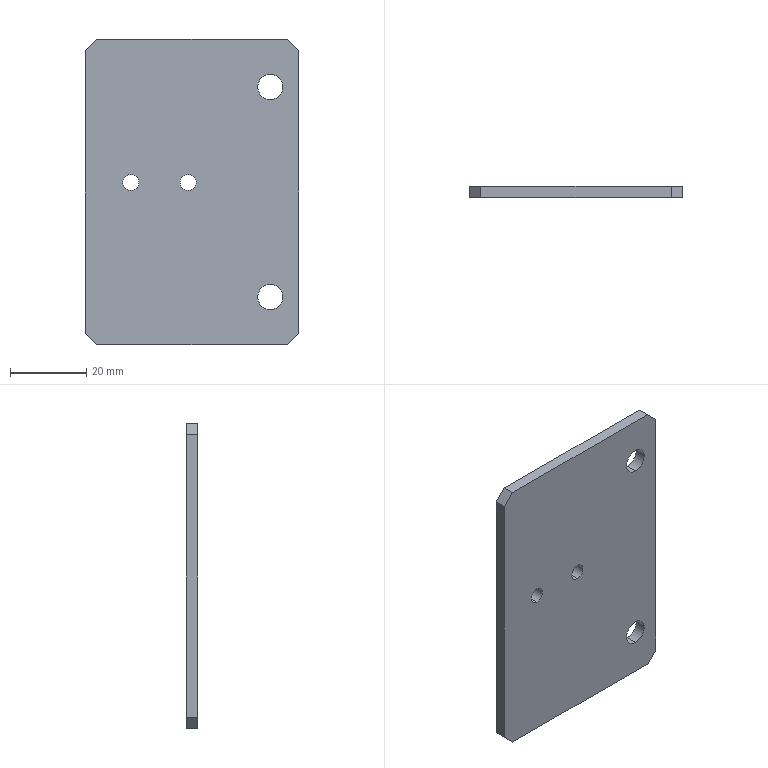Part | STEP file | 11-FG-SJ01311 | 1 solid | 18 faces | box 56 x 3 x 80 mm | volume 13098 mm3 | plane 10 | cylinder 8 | commonest cylinder face diameters 4.2 x4 6.6 x4
STEP:
#1=CARTESIAN_POINT('',(12.,50.,40.4));
#2=VERTEX_POINT('',#1);
#3=CARTESIAN_POINT('',(12.,50.,44.6));
#4=VERTEX_POINT('',#3);
#5=CARTESIAN_POINT('',(12.,50.,42.5));
#6=DIRECTION('',(0.,1.,0.));
#7=DIRECTION('',(0.,0.,1.));
#8=AXIS2_PLACEMENT_3D('',#5,#6,#7);
#9=CIRCLE('',#8,2.1);
#10=EDGE_CURVE('',#2,#4,#9,.T.);
#11=ORIENTED_EDGE('',*,*,#10,.T.);
#12=CARTESIAN_POINT('',(12.,47.,44.6));
#13=VERTEX_POINT('',#12);
#14=CARTESIAN_POINT('',(12.,47.,44.6));
#15=DIRECTION('',(0.,-1.,0.));
#16=VECTOR('',#15,1000.);
#17=LINE('',#14,#16);
#18=EDGE_CURVE('',#4,#13,#17,.T.);
#19=ORIENTED_EDGE('',*,*,#18,.T.);
#20=CARTESIAN_POINT('',(12.,47.,40.4));
#21=VERTEX_POINT('',#20);
#22=CARTESIAN_POINT('',(12.,47.,42.5));
#23=DIRECTION('',(0.,-1.,0.));
#24=DIRECTION('',(0.,0.,-1.));
#25=AXIS2_PLACEMENT_3D('',#22,#23,#24);
#26=CIRCLE('',#25,2.1);
#27=EDGE_CURVE('',#13,#21,#26,.T.);
#28=ORIENTED_EDGE('',*,*,#27,.T.);
#29=CARTESIAN_POINT('',(12.,47.,40.4));
#30=DIRECTION('',(0.,-1.,0.));
#31=VECTOR('',#30,1000.);
#32=LINE('',#29,#31);
#33=EDGE_CURVE('',#2,#21,#32,.T.);
#34=ORIENTED_EDGE('',*,*,#33,.F.);
#35=EDGE_LOOP('',(#11,#19,#28,#34));
#36=FACE_OUTER_BOUND('',#35,.T.);
#37=CARTESIAN_POINT('',(12.,47.,42.5));
#38=DIRECTION('',(0.,-1.,0.));
#39=DIRECTION('',(0.,0.,-1.));
#40=AXIS2_PLACEMENT_3D('',#37,#38,#39);
#41=CYLINDRICAL_SURFACE('',#40,2.1);
#42=ADVANCED_FACE('',(#36),#41,.F.);
#43=CARTESIAN_POINT('',(27.,50.,40.4));
#44=VERTEX_POINT('',#43);
#45=CARTESIAN_POINT('',(27.,50.,44.6));
#46=VERTEX_POINT('',#45);
#47=CARTESIAN_POINT('',(27.,50.,42.5));
#48=DIRECTION('',(0.,1.,0.));
#49=DIRECTION('',(0.,0.,1.));
#50=AXIS2_PLACEMENT_3D('',#47,#48,#49);
#51=CIRCLE('',#50,2.1);
#52=EDGE_CURVE('',#44,#46,#51,.T.);
#53=ORIENTED_EDGE('',*,*,#52,.T.);
#54=CARTESIAN_POINT('',(27.,47.,44.6));
#55=VERTEX_POINT('',#54);
#56=CARTESIAN_POINT('',(27.,47.,44.6));
#57=DIRECTION('',(0.,-1.,0.));
#58=VECTOR('',#57,1000.);
#59=LINE('',#56,#58);
#60=EDGE_CURVE('',#46,#55,#59,.T.);
#61=ORIENTED_EDGE('',*,*,#60,.T.);
#62=CARTESIAN_POINT('',(27.,47.,40.4));
#63=VERTEX_POINT('',#62);
#64=CARTESIAN_POINT('',(27.,47.,42.5));
#65=DIRECTION('',(0.,-1.,0.));
#66=DIRECTION('',(0.,0.,-1.));
#67=AXIS2_PLACEMENT_3D('',#64,#65,#66);
#68=CIRCLE('',#67,2.1);
#69=EDGE_CURVE('',#55,#63,#68,.T.);
#70=ORIENTED_EDGE('',*,*,#69,.T.);
#71=CARTESIAN_POINT('',(27.,47.,40.4));
#72=DIRECTION('',(0.,-1.,0.));
#73=VECTOR('',#72,1000.);
#74=LINE('',#71,#73);
#75=EDGE_CURVE('',#44,#63,#74,.T.);
#76=ORIENTED_EDGE('',*,*,#75,.F.);
#77=EDGE_LOOP('',(#53,#61,#70,#76));
#78=FACE_OUTER_BOUND('',#77,.T.);
#79=CARTESIAN_POINT('',(27.,47.,42.5));
#80=DIRECTION('',(0.,-1.,0.));
#81=DIRECTION('',(0.,0.,-1.));
#82=AXIS2_PLACEMENT_3D('',#79,#80,#81);
#83=CYLINDRICAL_SURFACE('',#82,2.1);
#84=ADVANCED_FACE('',(#78),#83,.F.);
#85=CARTESIAN_POINT('',(48.5,50.,70.8));
#86=VERTEX_POINT('',#85);
#87=CARTESIAN_POINT('',(48.5,50.,64.2));
#88=VERTEX_POINT('',#87);
#89=CARTESIAN_POINT('',(48.5,50.,67.5));
#90=DIRECTION('',(0.,-1.,0.));
#91=DIRECTION('',(0.,0.,-1.));
#92=AXIS2_PLACEMENT_3D('',#89,#90,#91);
#93=CIRCLE('',#92,3.3);
#94=EDGE_CURVE('',#86,#88,#93,.T.);
#95=ORIENTED_EDGE('',*,*,#94,.F.);
#96=CARTESIAN_POINT('',(48.5,47.,70.8));
#97=VERTEX_POINT('',#96);
#98=CARTESIAN_POINT('',(48.5,47.,70.8));
#99=DIRECTION('',(0.,-1.,0.));
#100=VECTOR('',#99,1000.);
#101=LINE('',#98,#100);
#102=EDGE_CURVE('',#86,#97,#101,.T.);
#103=ORIENTED_EDGE('',*,*,#102,.T.);
#104=CARTESIAN_POINT('',(48.5,47.,64.2));
#105=VERTEX_POINT('',#104);
#106=CARTESIAN_POINT('',(48.5,47.,67.5));
#107=DIRECTION('',(0.,-1.,0.));
#108=DIRECTION('',(0.,0.,-1.));
#109=AXIS2_PLACEMENT_3D('',#106,#107,#108);
#110=CIRCLE('',#109,3.3);
#111=EDGE_CURVE('',#97,#105,#110,.T.);
#112=ORIENTED_EDGE('',*,*,#111,.T.);
#113=CARTESIAN_POINT('',(48.5,47.,64.2));
#114=DIRECTION('',(0.,-1.,0.));
#115=VECTOR('',#114,1000.);
#116=LINE('',#113,#115);
#117=EDGE_CURVE('',#88,#105,#116,.T.);
#118=ORIENTED_EDGE('',*,*,#117,.F.);
#119=EDGE_LOOP('',(#95,#103,#112,#118));
#120=FACE_OUTER_BOUND('',#119,.T.);
#121=CARTESIAN_POINT('',(48.5,47.,67.5));
#122=DIRECTION('',(0.,-1.,0.));
#123=DIRECTION('',(0.,0.,-1.));
#124=AXIS2_PLACEMENT_3D('',#121,#122,#123);
#125=CYLINDRICAL_SURFACE('',#124,3.3);
#126=ADVANCED_FACE('',(#120),#125,.F.);
#127=CARTESIAN_POINT('',(48.5,50.,15.8));
#128=VERTEX_POINT('',#127);
#129=CARTESIAN_POINT('',(48.5,50.,9.2));
#130=VERTEX_POINT('',#129);
#131=CARTESIAN_POINT('',(48.5,50.,12.5));
#132=DIRECTION('',(0.,-1.,0.));
#133=DIRECTION('',(0.,0.,-1.));
#134=AXIS2_PLACEMENT_3D('',#131,#132,#133);
#135=CIRCLE('',#134,3.3);
#136=EDGE_CURVE('',#128,#130,#135,.T.);
#137=ORIENTED_EDGE('',*,*,#136,.F.);
#138=CARTESIAN_POINT('',(48.5,47.,15.8));
#139=VERTEX_POINT('',#138);
#140=CARTESIAN_POINT('',(48.5,47.,15.8));
#141=DIRECTION('',(0.,-1.,0.));
#142=VECTOR('',#141,1000.);
#143=LINE('',#140,#142);
#144=EDGE_CURVE('',#128,#139,#143,.T.);
#145=ORIENTED_EDGE('',*,*,#144,.T.);
#146=CARTESIAN_POINT('',(48.5,47.,9.2));
#147=VERTEX_POINT('',#146);
#148=CARTESIAN_POINT('',(48.5,47.,12.5));
#149=DIRECTION('',(0.,-1.,0.));
#150=DIRECTION('',(0.,0.,-1.));
#151=AXIS2_PLACEMENT_3D('',#148,#149,#150);
#152=CIRCLE('',#151,3.3);
#153=EDGE_CURVE('',#139,#147,#152,.T.);
#154=ORIENTED_EDGE('',*,*,#153,.T.);
#155=CARTESIAN_POINT('',(48.5,47.,9.2));
#156=DIRECTION('',(0.,-1.,0.));
#157=VECTOR('',#156,1000.);
#158=LINE('',#155,#157);
#159=EDGE_CURVE('',#130,#147,#158,.T.);
#160=ORIENTED_EDGE('',*,*,#159,.F.);
#161=EDGE_LOOP('',(#137,#145,#154,#160));
#162=FACE_OUTER_BOUND('',#161,.T.);
#163=CARTESIAN_POINT('',(48.5,47.,12.5));
#164=DIRECTION('',(0.,-1.,0.));
#165=DIRECTION('',(0.,0.,-1.));
#166=AXIS2_PLACEMENT_3D('',#163,#164,#165);
#167=CYLINDRICAL_SURFACE('',#166,3.3);
#168=ADVANCED_FACE('',(#162),#167,.F.);
#169=CARTESIAN_POINT('',(12.,47.,42.5));
#170=DIRECTION('',(0.,-1.,0.));
#171=DIRECTION('',(0.,0.,-1.));
#172=AXIS2_PLACEMENT_3D('',#169,#170,#171);
#173=CIRCLE('',#172,2.1);
#174=EDGE_CURVE('',#21,#13,#173,.T.);
#175=ORIENTED_EDGE('',*,*,#174,.F.);
#176=ORIENTED_EDGE('',*,*,#27,.F.);
#177=EDGE_LOOP('',(#175,#176));
#178=FACE_BOUND('',#177,.T.);
#179=CARTESIAN_POINT('',(27.,47.,42.5));
#180=DIRECTION('',(0.,-1.,0.));
#181=DIRECTION('',(0.,0.,-1.));
#182=AXIS2_PLACEMENT_3D('',#179,#180,#181);
#183=CIRCLE('',#182,2.1);
#184=EDGE_CURVE('',#63,#55,#183,.T.);
#185=ORIENTED_EDGE('',*,*,#184,.F.);
#186=ORIENTED_EDGE('',*,*,#69,.F.);
#187=EDGE_LOOP('',(#185,#186));
#188=FACE_BOUND('',#187,.T.);
#189=CARTESIAN_POINT('',(48.5,47.,67.5));
#190=DIRECTION('',(0.,-1.,0.));
#191=DIRECTION('',(0.,0.,-1.));
#192=AXIS2_PLACEMENT_3D('',#189,#190,#191);
#193=CIRCLE('',#192,3.3);
#194=EDGE_CURVE('',#105,#97,#193,.T.);
#195=ORIENTED_EDGE('',*,*,#194,.F.);
#196=ORIENTED_EDGE('',*,*,#111,.F.);
#197=EDGE_LOOP('',(#195,#196));
#198=FACE_BOUND('',#197,.T.);
#199=CARTESIAN_POINT('',(48.5,47.,12.5));
#200=DIRECTION('',(0.,-1.,0.));
#201=DIRECTION('',(0.,0.,-1.));
#202=AXIS2_PLACEMENT_3D('',#199,#200,#201);
#203=CIRCLE('',#202,3.3);
#204=EDGE_CURVE('',#147,#139,#203,.T.);
#205=ORIENTED_EDGE('',*,*,#204,.F.);
#206=ORIENTED_EDGE('',*,*,#153,.F.);
#207=EDGE_LOOP('',(#205,#206));
#208=FACE_BOUND('',#207,.T.);
#209=CARTESIAN_POINT('',(0.,47.,77.));
#210=VERTEX_POINT('',#209);
#211=CARTESIAN_POINT('',(0.,47.,3.));
#212=VERTEX_POINT('',#211);
#213=CARTESIAN_POINT('',(0.,47.,80.));
#214=DIRECTION('',(0.,0.,-1.));
#215=VECTOR('',#214,1000.);
#216=LINE('',#213,#215);
#217=EDGE_CURVE('',#210,#212,#216,.T.);
#218=ORIENTED_EDGE('',*,*,#217,.T.);
#219=CARTESIAN_POINT('',(3.,47.,0.));
#220=VERTEX_POINT('',#219);
#221=CARTESIAN_POINT('',(3.,47.,0.));
#222=DIRECTION('',(0.7071,0.,-0.7071));
#223=VECTOR('',#222,1000.);
#224=LINE('',#221,#223);
#225=EDGE_CURVE('',#212,#220,#224,.T.);
#226=ORIENTED_EDGE('',*,*,#225,.T.);
#227=CARTESIAN_POINT('',(53.,47.,0.));
#228=VERTEX_POINT('',#227);
#229=CARTESIAN_POINT('',(0.,47.,0.));
#230=DIRECTION('',(1.,0.,0.));
#231=VECTOR('',#230,1000.);
#232=LINE('',#229,#231);
#233=EDGE_CURVE('',#220,#228,#232,.T.);
#234=ORIENTED_EDGE('',*,*,#233,.T.);
#235=CARTESIAN_POINT('',(56.,47.,3.));
#236=VERTEX_POINT('',#235);
#237=CARTESIAN_POINT('',(53.,47.,0.));
#238=DIRECTION('',(0.7071,0.,0.7071));
#239=VECTOR('',#238,1000.);
#240=LINE('',#237,#239);
#241=EDGE_CURVE('',#228,#236,#240,.T.);
#242=ORIENTED_EDGE('',*,*,#241,.T.);
#243=CARTESIAN_POINT('',(56.,47.,77.));
#244=VERTEX_POINT('',#243);
#245=CARTESIAN_POINT('',(56.,47.,80.));
#246=DIRECTION('',(0.,0.,-1.));
#247=VECTOR('',#246,1000.);
#248=LINE('',#245,#247);
#249=EDGE_CURVE('',#244,#236,#248,.T.);
#250=ORIENTED_EDGE('',*,*,#249,.F.);
#251=CARTESIAN_POINT('',(53.,47.,80.));
#252=VERTEX_POINT('',#251);
#253=CARTESIAN_POINT('',(56.,47.,77.));
#254=DIRECTION('',(-0.7071,0.,0.7071));
#255=VECTOR('',#254,1000.);
#256=LINE('',#253,#255);
#257=EDGE_CURVE('',#244,#252,#256,.T.);
#258=ORIENTED_EDGE('',*,*,#257,.T.);
#259=CARTESIAN_POINT('',(3.,47.,80.));
#260=VERTEX_POINT('',#259);
#261=CARTESIAN_POINT('',(0.,47.,80.));
#262=DIRECTION('',(1.,0.,0.));
#263=VECTOR('',#262,1000.);
#264=LINE('',#261,#263);
#265=EDGE_CURVE('',#260,#252,#264,.T.);
#266=ORIENTED_EDGE('',*,*,#265,.F.);
#267=CARTESIAN_POINT('',(0.,47.,77.));
#268=DIRECTION('',(-0.7071,0.,-0.7071));
#269=VECTOR('',#268,1000.);
#270=LINE('',#267,#269);
#271=EDGE_CURVE('',#260,#210,#270,.T.);
#272=ORIENTED_EDGE('',*,*,#271,.T.);
#273=EDGE_LOOP('',(#218,#226,#234,#242,#250,#258,#266,#272));
#274=FACE_OUTER_BOUND('',#273,.T.);
#275=CARTESIAN_POINT('',(0.,47.,80.));
#276=DIRECTION('',(0.,1.,0.));
#277=DIRECTION('',(0.,0.,1.));
#278=AXIS2_PLACEMENT_3D('',#275,#276,#277);
#279=PLANE('',#278);
#280=ADVANCED_FACE('',(#178,#188,#198,#208,#274),#279,.F.);
#281=ORIENTED_EDGE('',*,*,#249,.T.);
#282=CARTESIAN_POINT('',(56.,50.,3.));
#283=VERTEX_POINT('',#282);
#284=CARTESIAN_POINT('',(56.,50.,3.));
#285=DIRECTION('',(0.,1.,0.));
#286=VECTOR('',#285,1000.);
#287=LINE('',#284,#286);
#288=EDGE_CURVE('',#236,#283,#287,.T.);
#289=ORIENTED_EDGE('',*,*,#288,.T.);
#290=CARTESIAN_POINT('',(56.,50.,77.));
#291=VERTEX_POINT('',#290);
#292=CARTESIAN_POINT('',(56.,50.,80.));
#293=DIRECTION('',(0.,0.,-1.));
#294=VECTOR('',#293,1000.);
#295=LINE('',#292,#294);
#296=EDGE_CURVE('',#291,#283,#295,.T.);
#297=ORIENTED_EDGE('',*,*,#296,.F.);
#298=CARTESIAN_POINT('',(56.,47.,77.));
#299=DIRECTION('',(0.,-1.,0.));
#300=VECTOR('',#299,1000.);
#301=LINE('',#298,#300);
#302=EDGE_CURVE('',#291,#244,#301,.T.);
#303=ORIENTED_EDGE('',*,*,#302,.T.);
#304=EDGE_LOOP('',(#281,#289,#297,#303));
#305=FACE_OUTER_BOUND('',#304,.T.);
#306=CARTESIAN_POINT('',(56.,50.,80.));
#307=DIRECTION('',(1.,0.,0.));
#308=DIRECTION('',(0.,0.,-1.));
#309=AXIS2_PLACEMENT_3D('',#306,#307,#308);
#310=PLANE('',#309);
#311=ADVANCED_FACE('',(#305),#310,.T.);
#312=ORIENTED_EDGE('',*,*,#10,.F.);
#313=CARTESIAN_POINT('',(12.,50.,42.5));
#314=DIRECTION('',(0.,1.,0.));
#315=DIRECTION('',(0.,0.,1.));
#316=AXIS2_PLACEMENT_3D('',#313,#314,#315);
#317=CIRCLE('',#316,2.1);
#318=EDGE_CURVE('',#4,#2,#317,.T.);
#319=ORIENTED_EDGE('',*,*,#318,.F.);
#320=EDGE_LOOP('',(#312,#319));
#321=FACE_BOUND('',#320,.T.);
#322=ORIENTED_EDGE('',*,*,#52,.F.);
#323=CARTESIAN_POINT('',(27.,50.,42.5));
#324=DIRECTION('',(0.,1.,0.));
#325=DIRECTION('',(0.,0.,1.));
#326=AXIS2_PLACEMENT_3D('',#323,#324,#325);
#327=CIRCLE('',#326,2.1);
#328=EDGE_CURVE('',#46,#44,#327,.T.);
#329=ORIENTED_EDGE('',*,*,#328,.F.);
#330=EDGE_LOOP('',(#322,#329));
#331=FACE_BOUND('',#330,.T.);
#332=CARTESIAN_POINT('',(48.5,50.,67.5));
#333=DIRECTION('',(0.,-1.,0.));
#334=DIRECTION('',(0.,0.,-1.));
#335=AXIS2_PLACEMENT_3D('',#332,#333,#334);
#336=CIRCLE('',#335,3.3);
#337=EDGE_CURVE('',#88,#86,#336,.T.);
#338=ORIENTED_EDGE('',*,*,#337,.T.);
#339=ORIENTED_EDGE('',*,*,#94,.T.);
#340=EDGE_LOOP('',(#338,#339));
#341=FACE_BOUND('',#340,.T.);
#342=CARTESIAN_POINT('',(48.5,50.,12.5));
#343=DIRECTION('',(0.,-1.,0.));
#344=DIRECTION('',(0.,0.,-1.));
#345=AXIS2_PLACEMENT_3D('',#342,#343,#344);
#346=CIRCLE('',#345,3.3);
#347=EDGE_CURVE('',#130,#128,#346,.T.);
#348=ORIENTED_EDGE('',*,*,#347,.T.);
#349=ORIENTED_EDGE('',*,*,#136,.T.);
#350=EDGE_LOOP('',(#348,#349));
#351=FACE_BOUND('',#350,.T.);
#352=CARTESIAN_POINT('',(3.,50.,0.));
#353=VERTEX_POINT('',#352);
#354=CARTESIAN_POINT('',(53.,50.,0.));
#355=VERTEX_POINT('',#354);
#356=CARTESIAN_POINT('',(0.,50.,0.));
#357=DIRECTION('',(1.,0.,0.));
#358=VECTOR('',#357,1000.);
#359=LINE('',#356,#358);
#360=EDGE_CURVE('',#353,#355,#359,.T.);
#361=ORIENTED_EDGE('',*,*,#360,.F.);
#362=CARTESIAN_POINT('',(0.,50.,3.));
#363=VERTEX_POINT('',#362);
#364=CARTESIAN_POINT('',(-38.5,50.,41.5));
#365=DIRECTION('',(-0.7071,0.,0.7071));
#366=VECTOR('',#365,1000.);
#367=LINE('',#364,#366);
#368=EDGE_CURVE('',#353,#363,#367,.T.);
#369=ORIENTED_EDGE('',*,*,#368,.T.);
#370=CARTESIAN_POINT('',(0.,50.,77.));
#371=VERTEX_POINT('',#370);
#372=CARTESIAN_POINT('',(0.,50.,80.));
#373=DIRECTION('',(0.,0.,-1.));
#374=VECTOR('',#373,1000.);
#375=LINE('',#372,#374);
#376=EDGE_CURVE('',#371,#363,#375,.T.);
#377=ORIENTED_EDGE('',*,*,#376,.F.);
#378=CARTESIAN_POINT('',(3.,50.,80.));
#379=VERTEX_POINT('',#378);
#380=CARTESIAN_POINT('',(1.5,50.,78.5));
#381=DIRECTION('',(0.7071,0.,0.7071));
#382=VECTOR('',#381,1000.);
#383=LINE('',#380,#382);
#384=EDGE_CURVE('',#371,#379,#383,.T.);
#385=ORIENTED_EDGE('',*,*,#384,.T.);
#386=CARTESIAN_POINT('',(53.,50.,80.));
#387=VERTEX_POINT('',#386);
#388=CARTESIAN_POINT('',(0.,50.,80.));
#389=DIRECTION('',(1.,0.,0.));
#390=VECTOR('',#389,1000.);
#391=LINE('',#388,#390);
#392=EDGE_CURVE('',#379,#387,#391,.T.);
#393=ORIENTED_EDGE('',*,*,#392,.T.);
#394=CARTESIAN_POINT('',(26.5,50.,106.5));
#395=DIRECTION('',(0.7071,0.,-0.7071));
#396=VECTOR('',#395,1000.);
#397=LINE('',#394,#396);
#398=EDGE_CURVE('',#387,#291,#397,.T.);
#399=ORIENTED_EDGE('',*,*,#398,.T.);
#400=ORIENTED_EDGE('',*,*,#296,.T.);
#401=CARTESIAN_POINT('',(66.5,50.,13.5));
#402=DIRECTION('',(-0.7071,0.,-0.7071));
#403=VECTOR('',#402,1000.);
#404=LINE('',#401,#403);
#405=EDGE_CURVE('',#283,#355,#404,.T.);
#406=ORIENTED_EDGE('',*,*,#405,.T.);
#407=EDGE_LOOP('',(#361,#369,#377,#385,#393,#399,#400,#406));
#408=FACE_OUTER_BOUND('',#407,.T.);
#409=CARTESIAN_POINT('',(0.,50.,80.));
#410=DIRECTION('',(0.,1.,0.));
#411=DIRECTION('',(0.,0.,1.));
#412=AXIS2_PLACEMENT_3D('',#409,#410,#411);
#413=PLANE('',#412);
#414=ADVANCED_FACE('',(#321,#331,#341,#351,#408),#413,.T.);
#415=ORIENTED_EDGE('',*,*,#376,.T.);
#416=CARTESIAN_POINT('',(0.,47.,3.));
#417=DIRECTION('',(0.,-1.,0.));
#418=VECTOR('',#417,1000.);
#419=LINE('',#416,#418);
#420=EDGE_CURVE('',#363,#212,#419,.T.);
#421=ORIENTED_EDGE('',*,*,#420,.T.);
#422=ORIENTED_EDGE('',*,*,#217,.F.);
#423=CARTESIAN_POINT('',(0.,50.,77.));
#424=DIRECTION('',(0.,1.,0.));
#425=VECTOR('',#424,1000.);
#426=LINE('',#423,#425);
#427=EDGE_CURVE('',#210,#371,#426,.T.);
#428=ORIENTED_EDGE('',*,*,#427,.T.);
#429=EDGE_LOOP('',(#415,#421,#422,#428));
#430=FACE_OUTER_BOUND('',#429,.T.);
#431=CARTESIAN_POINT('',(0.,47.,80.));
#432=DIRECTION('',(-1.,0.,0.));
#433=DIRECTION('',(0.,0.,1.));
#434=AXIS2_PLACEMENT_3D('',#431,#432,#433);
#435=PLANE('',#434);
#436=ADVANCED_FACE('',(#430),#435,.T.);
#437=ORIENTED_EDGE('',*,*,#392,.F.);
#438=CARTESIAN_POINT('',(3.,47.,80.));
#439=DIRECTION('',(0.,-1.,0.));
#440=VECTOR('',#439,1000.);
#441=LINE('',#438,#440);
#442=EDGE_CURVE('',#379,#260,#441,.T.);
#443=ORIENTED_EDGE('',*,*,#442,.T.);
#444=ORIENTED_EDGE('',*,*,#265,.T.);
#445=CARTESIAN_POINT('',(53.,50.,80.));
#446=DIRECTION('',(0.,1.,0.));
#447=VECTOR('',#446,1000.);
#448=LINE('',#445,#447);
#449=EDGE_CURVE('',#252,#387,#448,.T.);
#450=ORIENTED_EDGE('',*,*,#449,.T.);
#451=EDGE_LOOP('',(#437,#443,#444,#450));
#452=FACE_OUTER_BOUND('',#451,.T.);
#453=CARTESIAN_POINT('',(0.,0.,80.));
#454=DIRECTION('',(0.,0.,-1.));
#455=DIRECTION('',(-1.,0.,0.));
#456=AXIS2_PLACEMENT_3D('',#453,#454,#455);
#457=PLANE('',#456);
#458=ADVANCED_FACE('',(#452),#457,.F.);
#459=ORIENTED_EDGE('',*,*,#233,.F.);
#460=CARTESIAN_POINT('',(3.,0.,0.));
#461=DIRECTION('',(0.,1.,0.));
#462=VECTOR('',#461,1000.);
#463=LINE('',#460,#462);
#464=EDGE_CURVE('',#220,#353,#463,.T.);
#465=ORIENTED_EDGE('',*,*,#464,.T.);
#466=ORIENTED_EDGE('',*,*,#360,.T.);
#467=CARTESIAN_POINT('',(53.,0.,0.));
#468=DIRECTION('',(0.,-1.,0.));
#469=VECTOR('',#468,1000.);
#470=LINE('',#467,#469);
#471=EDGE_CURVE('',#355,#228,#470,.T.);
#472=ORIENTED_EDGE('',*,*,#471,.T.);
#473=EDGE_LOOP('',(#459,#465,#466,#472));
#474=FACE_OUTER_BOUND('',#473,.T.);
#475=CARTESIAN_POINT('',(0.,0.,0.));
#476=DIRECTION('',(0.,0.,-1.));
#477=DIRECTION('',(-1.,0.,0.));
#478=AXIS2_PLACEMENT_3D('',#475,#476,#477);
#479=PLANE('',#478);
#480=ADVANCED_FACE('',(#474),#479,.T.);
#481=ORIENTED_EDGE('',*,*,#225,.F.);
#482=ORIENTED_EDGE('',*,*,#420,.F.);
#483=ORIENTED_EDGE('',*,*,#368,.F.);
#484=ORIENTED_EDGE('',*,*,#464,.F.);
#485=EDGE_LOOP('',(#481,#482,#483,#484));
#486=FACE_OUTER_BOUND('',#485,.T.);
#487=CARTESIAN_POINT('',(3.,0.,0.));
#488=DIRECTION('',(0.7071,0.,0.7071));
#489=DIRECTION('',(0.,1.,0.));
#490=AXIS2_PLACEMENT_3D('',#487,#488,#489);
#491=PLANE('',#490);
#492=ADVANCED_FACE('',(#486),#491,.F.);
#493=ORIENTED_EDGE('',*,*,#271,.F.);
#494=ORIENTED_EDGE('',*,*,#442,.F.);
#495=ORIENTED_EDGE('',*,*,#384,.F.);
#496=ORIENTED_EDGE('',*,*,#427,.F.);
#497=EDGE_LOOP('',(#493,#494,#495,#496));
#498=FACE_OUTER_BOUND('',#497,.T.);
#499=CARTESIAN_POINT('',(0.,47.,77.));
#500=DIRECTION('',(-0.7071,0.,0.7071));
#501=DIRECTION('',(0.,-1.,0.));
#502=AXIS2_PLACEMENT_3D('',#499,#500,#501);
#503=PLANE('',#502);
#504=ADVANCED_FACE('',(#498),#503,.T.);
#505=ORIENTED_EDGE('',*,*,#405,.F.);
#506=ORIENTED_EDGE('',*,*,#288,.F.);
#507=ORIENTED_EDGE('',*,*,#241,.F.);
#508=ORIENTED_EDGE('',*,*,#471,.F.);
#509=EDGE_LOOP('',(#505,#506,#507,#508));
#510=FACE_OUTER_BOUND('',#509,.T.);
#511=CARTESIAN_POINT('',(53.,0.,0.));
#512=DIRECTION('',(-0.7071,0.,0.7071));
#513=DIRECTION('',(0.,-1.,0.));
#514=AXIS2_PLACEMENT_3D('',#511,#512,#513);
#515=PLANE('',#514);
#516=ADVANCED_FACE('',(#510),#515,.F.);
#517=ORIENTED_EDGE('',*,*,#398,.F.);
#518=ORIENTED_EDGE('',*,*,#449,.F.);
#519=ORIENTED_EDGE('',*,*,#257,.F.);
#520=ORIENTED_EDGE('',*,*,#302,.F.);
#521=EDGE_LOOP('',(#517,#518,#519,#520));
#522=FACE_OUTER_BOUND('',#521,.T.);
#523=CARTESIAN_POINT('',(56.,50.,77.));
#524=DIRECTION('',(0.7071,0.,0.7071));
#525=DIRECTION('',(0.,1.,0.));
#526=AXIS2_PLACEMENT_3D('',#523,#524,#525);
#527=PLANE('',#526);
#528=ADVANCED_FACE('',(#522),#527,.T.);
#529=ORIENTED_EDGE('',*,*,#144,.F.);
#530=ORIENTED_EDGE('',*,*,#347,.F.);
#531=ORIENTED_EDGE('',*,*,#159,.T.);
#532=ORIENTED_EDGE('',*,*,#204,.T.);
#533=EDGE_LOOP('',(#529,#530,#531,#532));
#534=FACE_OUTER_BOUND('',#533,.T.);
#535=CARTESIAN_POINT('',(48.5,47.,12.5));
#536=DIRECTION('',(0.,-1.,0.));
#537=DIRECTION('',(0.,0.,-1.));
#538=AXIS2_PLACEMENT_3D('',#535,#536,#537);
#539=CYLINDRICAL_SURFACE('',#538,3.3);
#540=ADVANCED_FACE('',(#534),#539,.F.);
#541=ORIENTED_EDGE('',*,*,#102,.F.);
#542=ORIENTED_EDGE('',*,*,#337,.F.);
#543=ORIENTED_EDGE('',*,*,#117,.T.);
#544=ORIENTED_EDGE('',*,*,#194,.T.);
#545=EDGE_LOOP('',(#541,#542,#543,#544));
#546=FACE_OUTER_BOUND('',#545,.T.);
#547=CARTESIAN_POINT('',(48.5,47.,67.5));
#548=DIRECTION('',(0.,-1.,0.));
#549=DIRECTION('',(0.,0.,-1.));
#550=AXIS2_PLACEMENT_3D('',#547,#548,#549);
#551=CYLINDRICAL_SURFACE('',#550,3.3);
#552=ADVANCED_FACE('',(#546),#551,.F.);
#553=ORIENTED_EDGE('',*,*,#60,.F.);
#554=ORIENTED_EDGE('',*,*,#328,.T.);
#555=ORIENTED_EDGE('',*,*,#75,.T.);
#556=ORIENTED_EDGE('',*,*,#184,.T.);
#557=EDGE_LOOP('',(#553,#554,#555,#556));
#558=FACE_OUTER_BOUND('',#557,.T.);
#559=CARTESIAN_POINT('',(27.,47.,42.5));
#560=DIRECTION('',(0.,-1.,0.));
#561=DIRECTION('',(0.,0.,-1.));
#562=AXIS2_PLACEMENT_3D('',#559,#560,#561);
#563=CYLINDRICAL_SURFACE('',#562,2.1);
#564=ADVANCED_FACE('',(#558),#563,.F.);
#565=ORIENTED_EDGE('',*,*,#18,.F.);
#566=ORIENTED_EDGE('',*,*,#318,.T.);
#567=ORIENTED_EDGE('',*,*,#33,.T.);
#568=ORIENTED_EDGE('',*,*,#174,.T.);
#569=EDGE_LOOP('',(#565,#566,#567,#568));
#570=FACE_OUTER_BOUND('',#569,.T.);
#571=CARTESIAN_POINT('',(12.,47.,42.5));
#572=DIRECTION('',(0.,-1.,0.));
#573=DIRECTION('',(0.,0.,-1.));
#574=AXIS2_PLACEMENT_3D('',#571,#572,#573);
#575=CYLINDRICAL_SURFACE('',#574,2.1);
#576=ADVANCED_FACE('',(#570),#575,.F.);
#577=CLOSED_SHELL('',(#42,#84,#126,#168,#280,#311,#414,#436,#458,#480,#492,#504,#516,#528,#540,#552,#564,#576));
#578=MANIFOLD_SOLID_BREP('',#577);
#579=CARTESIAN_POINT('',(0.,0.,0.));
#580=DIRECTION('',(0.,0.,1.));
#581=DIRECTION('',(1.,0.,0.));
#582=AXIS2_PLACEMENT_3D('',#579,#580,#581);
#583=(LENGTH_UNIT()NAMED_UNIT(*)SI_UNIT(.MILLI.,.METRE.));
#584=UNCERTAINTY_MEASURE_WITH_UNIT(LENGTH_MEASURE(0.00001),#583,'','');
#585=(NAMED_UNIT(*)PLANE_ANGLE_UNIT()SI_UNIT($,.RADIAN.));
#586=(NAMED_UNIT(*)SI_UNIT($,.STERADIAN.)SOLID_ANGLE_UNIT());
#587=(GEOMETRIC_REPRESENTATION_CONTEXT(3)GLOBAL_UNCERTAINTY_ASSIGNED_CONTEXT((#584))GLOBAL_UNIT_ASSIGNED_CONTEXT((#583,#585,#586))REPRESENTATION_CONTEXT('',''));
#588=ADVANCED_BREP_SHAPE_REPRESENTATION('',(#578,#582),#587);